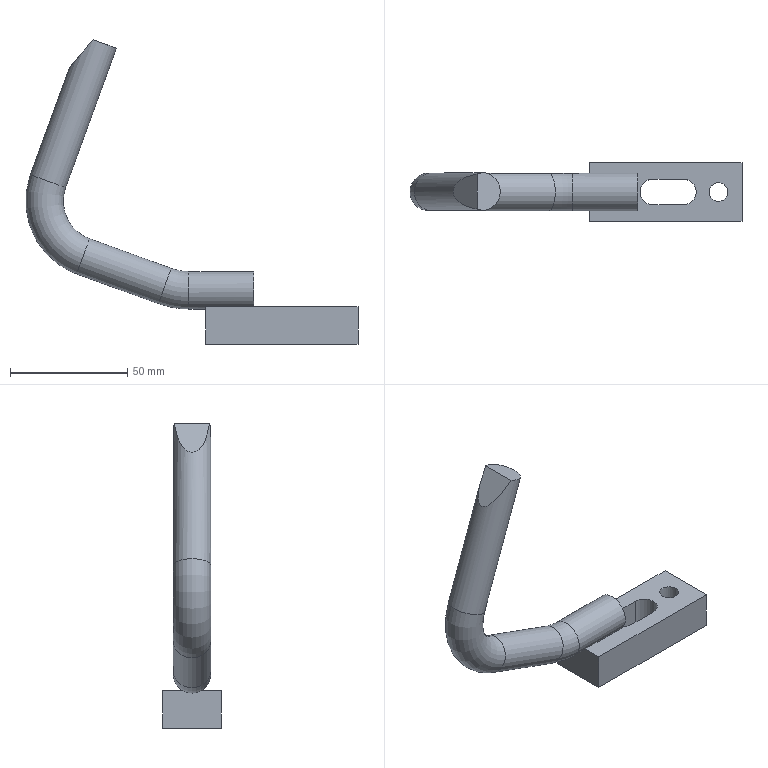Part | NX | features MAIN_BODY 2 | 1 solid | 19 faces | box 141.738 x 25 x 129.841 mm | volume 56656 mm3 | plane 10 | cylinder 6 | torus 2 | spline 1 | commonest cylinder face diameters 16 x3 11 x2 8 x1
STEP:
#1=CARTESIAN_POINT('',(970.,-301.373,-139.));
#2=VERTEX_POINT('',#1);
#3=CARTESIAN_POINT('',(970.,-293.627,-139.));
#4=VERTEX_POINT('',#3);
#5=CARTESIAN_POINT('',(970.,-297.5,-132.));
#6=DIRECTION('',(-1.,0.,0.));
#7=DIRECTION('',(0.,-1.,0.));
#8=AXIS2_PLACEMENT_3D('',#5,#6,#7);
#9=CIRCLE('',#8,8.);
#10=EDGE_CURVE('',#2,#4,#9,.F.);
#11=ORIENTED_EDGE('',*,*,#10,.T.);
#12=CARTESIAN_POINT('',(970.,-285.,-139.));
#13=VERTEX_POINT('',#12);
#14=CARTESIAN_POINT('',(970.,-285.5,-139.));
#15=DIRECTION('',(0.,1.,0.));
#16=VECTOR('',#15,1000.);
#17=LINE('',#14,#16);
#18=EDGE_CURVE('',#13,#4,#17,.F.);
#19=ORIENTED_EDGE('',*,*,#18,.F.);
#20=CARTESIAN_POINT('',(970.,-285.,-155.));
#21=VERTEX_POINT('',#20);
#22=CARTESIAN_POINT('',(970.,-285.,-135.));
#23=DIRECTION('',(0.,0.,-1.));
#24=VECTOR('',#23,1000.);
#25=LINE('',#22,#24);
#26=EDGE_CURVE('',#21,#13,#25,.F.);
#27=ORIENTED_EDGE('',*,*,#26,.F.);
#28=CARTESIAN_POINT('',(970.,-310.,-155.));
#29=VERTEX_POINT('',#28);
#30=CARTESIAN_POINT('',(970.,-285.5,-155.));
#31=DIRECTION('',(0.,1.,0.));
#32=VECTOR('',#31,1000.);
#33=LINE('',#30,#32);
#34=EDGE_CURVE('',#21,#29,#33,.F.);
#35=ORIENTED_EDGE('',*,*,#34,.T.);
#36=CARTESIAN_POINT('',(970.,-310.,-139.));
#37=VERTEX_POINT('',#36);
#38=CARTESIAN_POINT('',(970.,-310.,-135.));
#39=DIRECTION('',(0.,0.,1.));
#40=VECTOR('',#39,1000.);
#41=LINE('',#38,#40);
#42=EDGE_CURVE('',#29,#37,#41,.T.);
#43=ORIENTED_EDGE('',*,*,#42,.T.);
#44=CARTESIAN_POINT('',(970.,-285.5,-139.));
#45=DIRECTION('',(0.,1.,0.));
#46=VECTOR('',#45,1000.);
#47=LINE('',#44,#46);
#48=EDGE_CURVE('',#2,#37,#47,.F.);
#49=ORIENTED_EDGE('',*,*,#48,.F.);
#50=EDGE_LOOP('',(#11,#19,#27,#35,#43,#49));
#51=FACE_BOUND('',#50,.T.);
#52=CARTESIAN_POINT('',(970.,-285.5,-135.));
#53=DIRECTION('',(1.,0.,0.));
#54=DIRECTION('',(0.,-1.,0.));
#55=AXIS2_PLACEMENT_3D('',#52,#53,#54);
#56=PLANE('',#55);
#57=ADVANCED_FACE('',(#51),#56,.F.);
#58=ORIENTED_EDGE('',*,*,#48,.T.);
#59=CARTESIAN_POINT('',(1035.,-310.,-139.));
#60=VERTEX_POINT('',#59);
#61=CARTESIAN_POINT('',(900.,-310.,-139.));
#62=DIRECTION('',(-1.,0.,0.));
#63=VECTOR('',#62,1000.);
#64=LINE('',#61,#63);
#65=EDGE_CURVE('',#37,#60,#64,.F.);
#66=ORIENTED_EDGE('',*,*,#65,.T.);
#67=CARTESIAN_POINT('',(1035.,-285.,-139.));
#68=VERTEX_POINT('',#67);
#69=CARTESIAN_POINT('',(1035.,-285.5,-139.));
#70=DIRECTION('',(0.,-1.,0.));
#71=VECTOR('',#70,1000.);
#72=LINE('',#69,#71);
#73=EDGE_CURVE('',#68,#60,#72,.T.);
#74=ORIENTED_EDGE('',*,*,#73,.F.);
#75=CARTESIAN_POINT('',(900.,-285.,-139.));
#76=DIRECTION('',(1.,0.,0.));
#77=VECTOR('',#76,1000.);
#78=LINE('',#75,#77);
#79=EDGE_CURVE('',#13,#68,#78,.T.);
#80=ORIENTED_EDGE('',*,*,#79,.F.);
#81=ORIENTED_EDGE('',*,*,#18,.T.);
#82=CARTESIAN_POINT('',(990.552,-293.627,-139.));
#83=VERTEX_POINT('',#82);
#84=CARTESIAN_POINT('',(962.842,-293.627,-139.));
#85=DIRECTION('',(1.,0.,0.));
#86=VECTOR('',#85,1000.);
#87=LINE('',#84,#86);
#88=EDGE_CURVE('',#83,#4,#87,.F.);
#89=ORIENTED_EDGE('',*,*,#88,.F.);
#90=CARTESIAN_POINT('',(990.552,-301.373,-139.));
#91=VERTEX_POINT('',#90);
#92=CARTESIAN_POINT('',(990.552,-285.5,-139.));
#93=DIRECTION('',(0.,1.,0.));
#94=VECTOR('',#93,1000.);
#95=LINE('',#92,#94);
#96=EDGE_CURVE('',#91,#83,#95,.T.);
#97=ORIENTED_EDGE('',*,*,#96,.F.);
#98=CARTESIAN_POINT('',(962.842,-301.373,-139.));
#99=DIRECTION('',(1.,0.,0.));
#100=VECTOR('',#99,1000.);
#101=LINE('',#98,#100);
#102=EDGE_CURVE('',#2,#91,#101,.T.);
#103=ORIENTED_EDGE('',*,*,#102,.F.);
#104=EDGE_LOOP('',(#58,#66,#74,#80,#81,#89,#97,#103));
#105=FACE_BOUND('',#104,.T.);
#106=CARTESIAN_POINT('',(1021.,-297.5,-139.));
#107=VERTEX_POINT('',#106);
#108=CARTESIAN_POINT('',(1025.,-297.5,-139.));
#109=DIRECTION('',(0.,0.,1.));
#110=DIRECTION('',(-1.,0.,0.));
#111=AXIS2_PLACEMENT_3D('',#108,#109,#110);
#112=CIRCLE('',#111,4.);
#113=EDGE_CURVE('',#107,#107,#112,.F.);
#114=ORIENTED_EDGE('',*,*,#113,.T.);
#115=EDGE_LOOP('',(#114));
#116=FACE_BOUND('',#115,.T.);
#117=CARTESIAN_POINT('',(1010.,-292.,-139.));
#118=VERTEX_POINT('',#117);
#119=CARTESIAN_POINT('',(1010.,-303.,-139.));
#120=VERTEX_POINT('',#119);
#121=CARTESIAN_POINT('',(1010.,-297.5,-139.));
#122=DIRECTION('',(0.,0.,1.));
#123=DIRECTION('',(-1.,0.,0.));
#124=AXIS2_PLACEMENT_3D('',#121,#122,#123);
#125=CIRCLE('',#124,5.5);
#126=EDGE_CURVE('',#118,#120,#125,.F.);
#127=ORIENTED_EDGE('',*,*,#126,.T.);
#128=CARTESIAN_POINT('',(997.,-303.,-139.));
#129=VERTEX_POINT('',#128);
#130=CARTESIAN_POINT('',(969.,-303.,-139.));
#131=DIRECTION('',(-1.,0.,0.));
#132=VECTOR('',#131,1000.);
#133=LINE('',#130,#132);
#134=EDGE_CURVE('',#120,#129,#133,.T.);
#135=ORIENTED_EDGE('',*,*,#134,.T.);
#136=CARTESIAN_POINT('',(997.,-292.,-139.));
#137=VERTEX_POINT('',#136);
#138=CARTESIAN_POINT('',(997.,-297.5,-139.));
#139=DIRECTION('',(0.,0.,1.));
#140=DIRECTION('',(-1.,0.,0.));
#141=AXIS2_PLACEMENT_3D('',#138,#139,#140);
#142=CIRCLE('',#141,5.5);
#143=EDGE_CURVE('',#129,#137,#142,.F.);
#144=ORIENTED_EDGE('',*,*,#143,.T.);
#145=CARTESIAN_POINT('',(969.,-292.,-139.));
#146=DIRECTION('',(-1.,0.,0.));
#147=VECTOR('',#146,1000.);
#148=LINE('',#145,#147);
#149=EDGE_CURVE('',#137,#118,#148,.F.);
#150=ORIENTED_EDGE('',*,*,#149,.T.);
#151=EDGE_LOOP('',(#127,#135,#144,#150));
#152=FACE_BOUND('',#151,.T.);
#153=CARTESIAN_POINT('',(900.,-285.5,-139.));
#154=DIRECTION('',(0.,0.,-1.));
#155=DIRECTION('',(-1.,0.,0.));
#156=AXIS2_PLACEMENT_3D('',#153,#154,#155);
#157=PLANE('',#156);
#158=ADVANCED_FACE('',(#105,#116,#152),#157,.F.);
#159=CARTESIAN_POINT('',(1035.,-285.,-155.));
#160=VERTEX_POINT('',#159);
#161=CARTESIAN_POINT('',(1035.,-285.,-135.));
#162=DIRECTION('',(0.,0.,1.));
#163=VECTOR('',#162,1000.);
#164=LINE('',#161,#163);
#165=EDGE_CURVE('',#160,#68,#164,.T.);
#166=ORIENTED_EDGE('',*,*,#165,.F.);
#167=CARTESIAN_POINT('',(900.,-285.,-155.));
#168=DIRECTION('',(1.,0.,0.));
#169=VECTOR('',#168,1000.);
#170=LINE('',#167,#169);
#171=EDGE_CURVE('',#21,#160,#170,.T.);
#172=ORIENTED_EDGE('',*,*,#171,.F.);
#173=ORIENTED_EDGE('',*,*,#26,.T.);
#174=ORIENTED_EDGE('',*,*,#79,.T.);
#175=EDGE_LOOP('',(#166,#172,#173,#174));
#176=FACE_BOUND('',#175,.T.);
#177=CARTESIAN_POINT('',(900.,-285.,-135.));
#178=DIRECTION('',(0.,1.,0.));
#179=DIRECTION('',(1.,0.,0.));
#180=AXIS2_PLACEMENT_3D('',#177,#178,#179);
#181=PLANE('',#180);
#182=ADVANCED_FACE('',(#176),#181,.T.);
#183=ORIENTED_EDGE('',*,*,#42,.F.);
#184=CARTESIAN_POINT('',(1035.,-310.,-155.));
#185=VERTEX_POINT('',#184);
#186=CARTESIAN_POINT('',(900.,-310.,-155.));
#187=DIRECTION('',(-1.,0.,0.));
#188=VECTOR('',#187,1000.);
#189=LINE('',#186,#188);
#190=EDGE_CURVE('',#29,#185,#189,.F.);
#191=ORIENTED_EDGE('',*,*,#190,.T.);
#192=CARTESIAN_POINT('',(1035.,-310.,-135.));
#193=DIRECTION('',(0.,0.,-1.));
#194=VECTOR('',#193,1000.);
#195=LINE('',#192,#194);
#196=EDGE_CURVE('',#185,#60,#195,.F.);
#197=ORIENTED_EDGE('',*,*,#196,.T.);
#198=ORIENTED_EDGE('',*,*,#65,.F.);
#199=EDGE_LOOP('',(#183,#191,#197,#198));
#200=FACE_BOUND('',#199,.T.);
#201=CARTESIAN_POINT('',(900.,-310.,-135.));
#202=DIRECTION('',(0.,1.,0.));
#203=DIRECTION('',(1.,0.,0.));
#204=AXIS2_PLACEMENT_3D('',#201,#202,#203);
#205=PLANE('',#204);
#206=ADVANCED_FACE('',(#200),#205,.F.);
#207=CARTESIAN_POINT('',(1035.,-285.5,-155.));
#208=DIRECTION('',(0.,-1.,0.));
#209=VECTOR('',#208,1000.);
#210=LINE('',#207,#209);
#211=EDGE_CURVE('',#160,#185,#210,.T.);
#212=ORIENTED_EDGE('',*,*,#211,.F.);
#213=ORIENTED_EDGE('',*,*,#165,.T.);
#214=ORIENTED_EDGE('',*,*,#73,.T.);
#215=ORIENTED_EDGE('',*,*,#196,.F.);
#216=EDGE_LOOP('',(#212,#213,#214,#215));
#217=FACE_BOUND('',#216,.T.);
#218=CARTESIAN_POINT('',(1035.,-285.5,-135.));
#219=DIRECTION('',(1.,0.,0.));
#220=DIRECTION('',(0.,-1.,0.));
#221=AXIS2_PLACEMENT_3D('',#218,#219,#220);
#222=PLANE('',#221);
#223=ADVANCED_FACE('',(#217),#222,.T.);
#224=CARTESIAN_POINT('',(1021.03,-297.987,-155.));
#225=VERTEX_POINT('',#224);
#226=CARTESIAN_POINT('',(1025.,-297.5,-155.));
#227=DIRECTION('',(0.,0.,-1.));
#228=DIRECTION('',(-0.9925,-0.1219,0.));
#229=AXIS2_PLACEMENT_3D('',#226,#227,#228);
#230=CIRCLE('',#229,4.);
#231=EDGE_CURVE('',#225,#225,#230,.T.);
#232=ORIENTED_EDGE('',*,*,#231,.F.);
#233=EDGE_LOOP('',(#232));
#234=FACE_BOUND('',#233,.T.);
#235=CARTESIAN_POINT('',(1010.,-303.,-155.));
#236=VERTEX_POINT('',#235);
#237=CARTESIAN_POINT('',(997.,-303.,-155.));
#238=VERTEX_POINT('',#237);
#239=CARTESIAN_POINT('',(969.,-303.,-155.));
#240=DIRECTION('',(-1.,0.,0.));
#241=VECTOR('',#240,1000.);
#242=LINE('',#239,#241);
#243=EDGE_CURVE('',#236,#238,#242,.T.);
#244=ORIENTED_EDGE('',*,*,#243,.F.);
#245=CARTESIAN_POINT('',(1010.,-292.,-155.));
#246=VERTEX_POINT('',#245);
#247=CARTESIAN_POINT('',(1010.,-297.5,-155.));
#248=DIRECTION('',(0.,0.,1.));
#249=DIRECTION('',(-0.9925,-0.1219,0.));
#250=AXIS2_PLACEMENT_3D('',#247,#248,#249);
#251=CIRCLE('',#250,5.5);
#252=EDGE_CURVE('',#246,#236,#251,.F.);
#253=ORIENTED_EDGE('',*,*,#252,.F.);
#254=CARTESIAN_POINT('',(997.,-292.,-155.));
#255=VERTEX_POINT('',#254);
#256=CARTESIAN_POINT('',(969.,-292.,-155.));
#257=DIRECTION('',(-1.,0.,0.));
#258=VECTOR('',#257,1000.);
#259=LINE('',#256,#258);
#260=EDGE_CURVE('',#255,#246,#259,.F.);
#261=ORIENTED_EDGE('',*,*,#260,.F.);
#262=CARTESIAN_POINT('',(997.,-297.5,-155.));
#263=DIRECTION('',(0.,0.,1.));
#264=DIRECTION('',(-0.9925,-0.1219,0.));
#265=AXIS2_PLACEMENT_3D('',#262,#263,#264);
#266=CIRCLE('',#265,5.5);
#267=EDGE_CURVE('',#238,#255,#266,.F.);
#268=ORIENTED_EDGE('',*,*,#267,.F.);
#269=EDGE_LOOP('',(#244,#253,#261,#268));
#270=FACE_BOUND('',#269,.T.);
#271=ORIENTED_EDGE('',*,*,#190,.F.);
#272=ORIENTED_EDGE('',*,*,#34,.F.);
#273=ORIENTED_EDGE('',*,*,#171,.T.);
#274=ORIENTED_EDGE('',*,*,#211,.T.);
#275=EDGE_LOOP('',(#271,#272,#273,#274));
#276=FACE_BOUND('',#275,.T.);
#277=CARTESIAN_POINT('',(900.,-285.5,-155.));
#278=DIRECTION('',(0.,0.,-1.));
#279=DIRECTION('',(-1.,0.,0.));
#280=AXIS2_PLACEMENT_3D('',#277,#278,#279);
#281=PLANE('',#280);
#282=ADVANCED_FACE('',(#234,#270,#276),#281,.T.);
#283=ORIENTED_EDGE('',*,*,#143,.F.);
#284=CARTESIAN_POINT('',(997.,-303.,-119.));
#285=DIRECTION('',(0.,0.,-1.));
#286=VECTOR('',#285,1000.);
#287=LINE('',#284,#286);
#288=EDGE_CURVE('',#129,#238,#287,.T.);
#289=ORIENTED_EDGE('',*,*,#288,.T.);
#290=ORIENTED_EDGE('',*,*,#267,.T.);
#291=CARTESIAN_POINT('',(997.,-292.,-119.));
#292=DIRECTION('',(0.,0.,-1.));
#293=VECTOR('',#292,1000.);
#294=LINE('',#291,#293);
#295=EDGE_CURVE('',#137,#255,#294,.T.);
#296=ORIENTED_EDGE('',*,*,#295,.F.);
#297=EDGE_LOOP('',(#283,#289,#290,#296));
#298=FACE_BOUND('',#297,.T.);
#299=CARTESIAN_POINT('',(997.,-297.5,-119.));
#300=DIRECTION('',(0.,0.,-1.));
#301=DIRECTION('',(-1.,0.,0.));
#302=AXIS2_PLACEMENT_3D('',#299,#300,#301);
#303=CYLINDRICAL_SURFACE('',#302,5.5);
#304=ADVANCED_FACE('',(#298),#303,.F.);
#305=ORIENTED_EDGE('',*,*,#126,.F.);
#306=CARTESIAN_POINT('',(1010.,-292.,-119.));
#307=DIRECTION('',(0.,0.,-1.));
#308=VECTOR('',#307,1000.);
#309=LINE('',#306,#308);
#310=EDGE_CURVE('',#118,#246,#309,.T.);
#311=ORIENTED_EDGE('',*,*,#310,.T.);
#312=ORIENTED_EDGE('',*,*,#252,.T.);
#313=CARTESIAN_POINT('',(1010.,-303.,-119.));
#314=DIRECTION('',(0.,0.,-1.));
#315=VECTOR('',#314,1000.);
#316=LINE('',#313,#315);
#317=EDGE_CURVE('',#120,#236,#316,.T.);
#318=ORIENTED_EDGE('',*,*,#317,.F.);
#319=EDGE_LOOP('',(#305,#311,#312,#318));
#320=FACE_BOUND('',#319,.T.);
#321=CARTESIAN_POINT('',(1010.,-297.5,-119.));
#322=DIRECTION('',(0.,0.,-1.));
#323=DIRECTION('',(-1.,0.,0.));
#324=AXIS2_PLACEMENT_3D('',#321,#322,#323);
#325=CYLINDRICAL_SURFACE('',#324,5.5);
#326=ADVANCED_FACE('',(#320),#325,.F.);
#327=ORIENTED_EDGE('',*,*,#317,.T.);
#328=ORIENTED_EDGE('',*,*,#243,.T.);
#329=ORIENTED_EDGE('',*,*,#288,.F.);
#330=ORIENTED_EDGE('',*,*,#134,.F.);
#331=EDGE_LOOP('',(#327,#328,#329,#330));
#332=FACE_BOUND('',#331,.T.);
#333=CARTESIAN_POINT('',(969.,-303.,-119.));
#334=DIRECTION('',(0.,-1.,0.));
#335=DIRECTION('',(-1.,0.,0.));
#336=AXIS2_PLACEMENT_3D('',#333,#334,#335);
#337=PLANE('',#336);
#338=ADVANCED_FACE('',(#332),#337,.F.);
#339=ORIENTED_EDGE('',*,*,#295,.T.);
#340=ORIENTED_EDGE('',*,*,#260,.T.);
#341=ORIENTED_EDGE('',*,*,#310,.F.);
#342=ORIENTED_EDGE('',*,*,#149,.F.);
#343=EDGE_LOOP('',(#339,#340,#341,#342));
#344=FACE_BOUND('',#343,.T.);
#345=CARTESIAN_POINT('',(969.,-292.,-119.));
#346=DIRECTION('',(0.,-1.,0.));
#347=DIRECTION('',(-1.,0.,0.));
#348=AXIS2_PLACEMENT_3D('',#345,#346,#347);
#349=PLANE('',#348);
#350=ADVANCED_FACE('',(#344),#349,.T.);
#351=ORIENTED_EDGE('',*,*,#231,.T.);
#352=EDGE_LOOP('',(#351));
#353=FACE_BOUND('',#352,.T.);
#354=ORIENTED_EDGE('',*,*,#113,.F.);
#355=EDGE_LOOP('',(#354));
#356=FACE_BOUND('',#355,.T.);
#357=CARTESIAN_POINT('',(1025.,-297.5,-139.));
#358=DIRECTION('',(0.,0.,-1.));
#359=DIRECTION('',(-0.9925,-0.1219,0.));
#360=AXIS2_PLACEMENT_3D('',#357,#358,#359);
#361=CYLINDRICAL_SURFACE('',#360,4.);
#362=ADVANCED_FACE('',(#353,#356),#361,.F.);
#363=CARTESIAN_POINT('',(962.842,-297.5,-140.));
#364=VERTEX_POINT('',#363);
#365=CARTESIAN_POINT('',(962.842,-297.5,-132.));
#366=DIRECTION('',(-1.,0.,0.));
#367=DIRECTION('',(0.,0.,-1.));
#368=AXIS2_PLACEMENT_3D('',#365,#366,#367);
#369=CIRCLE('',#368,8.);
#370=EDGE_CURVE('',#364,#364,#369,.T.);
#371=ORIENTED_EDGE('',*,*,#370,.F.);
#372=EDGE_LOOP('',(#371));
#373=FACE_BOUND('',#372,.T.);
#374=ORIENTED_EDGE('',*,*,#102,.T.);
#375=CARTESIAN_POINT('',(990.552,-297.5,-132.));
#376=DIRECTION('',(-1.,0.,0.));
#377=DIRECTION('',(0.,0.,-1.));
#378=AXIS2_PLACEMENT_3D('',#375,#376,#377);
#379=CIRCLE('',#378,8.);
#380=EDGE_CURVE('',#91,#83,#379,.T.);
#381=ORIENTED_EDGE('',*,*,#380,.T.);
#382=ORIENTED_EDGE('',*,*,#88,.T.);
#383=ORIENTED_EDGE('',*,*,#10,.F.);
#384=EDGE_LOOP('',(#374,#381,#382,#383));
#385=FACE_BOUND('',#384,.T.);
#386=CARTESIAN_POINT('',(962.842,-297.5,-132.));
#387=DIRECTION('',(1.,0.,0.));
#388=DIRECTION('',(0.,0.,-1.));
#389=AXIS2_PLACEMENT_3D('',#386,#387,#388);
#390=CYLINDRICAL_SURFACE('',#389,8.);
#391=ADVANCED_FACE('',(#373,#385),#390,.T.);
#392=ORIENTED_EDGE('',*,*,#96,.T.);
#393=ORIENTED_EDGE('',*,*,#380,.F.);
#394=EDGE_LOOP('',(#392,#393));
#395=FACE_BOUND('',#394,.T.);
#396=CARTESIAN_POINT('',(990.552,-297.5,-132.));
#397=DIRECTION('',(1.,0.,0.));
#398=DIRECTION('',(0.,0.,-1.));
#399=AXIS2_PLACEMENT_3D('',#396,#397,#398);
#400=PLANE('',#399);
#401=ADVANCED_FACE('',(#395),#400,.T.);
#402=CARTESIAN_POINT('',(895.252,-297.5,-82.72));
#403=VERTEX_POINT('',#402);
#404=CARTESIAN_POINT('',(902.769,-297.5,-85.456));
#405=DIRECTION('',(0.342,0.,0.9397));
#406=DIRECTION('',(-0.9397,0.,0.342));
#407=AXIS2_PLACEMENT_3D('',#404,#405,#406);
#408=CIRCLE('',#407,8.);
#409=EDGE_CURVE('',#403,#403,#408,.T.);
#410=ORIENTED_EDGE('',*,*,#409,.T.);
#411=EDGE_LOOP('',(#410));
#412=FACE_BOUND('',#411,.T.);
#413=CARTESIAN_POINT('',(921.975,-305.074,-25.159));
#414=VERTEX_POINT('',#413);
#415=CARTESIAN_POINT('',(921.975,-289.926,-25.159));
#416=VERTEX_POINT('',#415);
#417=CARTESIAN_POINT('',(924.395,-297.5,-26.04));
#418=DIRECTION('',(0.342,0.,0.9397));
#419=DIRECTION('',(-0.9397,0.,0.342));
#420=AXIS2_PLACEMENT_3D('',#417,#418,#419);
#421=CIRCLE('',#420,8.);
#422=EDGE_CURVE('',#414,#416,#421,.T.);
#423=ORIENTED_EDGE('',*,*,#422,.F.);
#424=CARTESIAN_POINT('',(921.975,-289.926,-25.159));
#425=CARTESIAN_POINT('',(920.983,-290.105,-26.342));
#426=CARTESIAN_POINT('',(919.015,-290.582,-28.686));
#427=CARTESIAN_POINT('',(916.59,-291.561,-31.577));
#428=CARTESIAN_POINT('',(914.734,-292.685,-33.788));
#429=CARTESIAN_POINT('',(913.406,-293.799,-35.371));
#430=CARTESIAN_POINT('',(912.229,-295.253,-36.773));
#431=CARTESIAN_POINT('',(911.548,-297.538,-37.585));
#432=CARTESIAN_POINT('',(912.262,-299.8,-36.734));
#433=CARTESIAN_POINT('',(913.447,-301.242,-35.323));
#434=CARTESIAN_POINT('',(914.775,-302.342,-33.739));
#435=CARTESIAN_POINT('',(916.614,-303.449,-31.547));
#436=CARTESIAN_POINT('',(919.022,-304.419,-28.679));
#437=CARTESIAN_POINT('',(920.987,-304.895,-26.336));
#438=CARTESIAN_POINT('',(921.975,-305.074,-25.159));
#439=B_SPLINE_CURVE_WITH_KNOTS('',3,(#424,#425,#426,#427,#428,#429,#430,#431,#432,#433,#434,#435,#436,#437,#438),.UNSPECIFIED.,.F.,.F.,(4,1,1,1,1,1,1,1,1,1,1,1,4),(0.,0.004649,0.009299,0.01162,0.01395,0.01627,0.0186,0.02092,0.02325,0.02557,0.0279,0.03255,0.03719),.UNSPECIFIED.);
#440=EDGE_CURVE('',#416,#414,#439,.T.);
#441=ORIENTED_EDGE('',*,*,#440,.F.);
#442=EDGE_LOOP('',(#423,#441));
#443=FACE_BOUND('',#442,.T.);
#444=CARTESIAN_POINT('',(902.769,-297.5,-85.456));
#445=DIRECTION('',(0.342,0.,0.9397));
#446=DIRECTION('',(0.9397,0.,-0.342));
#447=AXIS2_PLACEMENT_3D('',#444,#445,#446);
#448=CYLINDRICAL_SURFACE('',#447,8.);
#449=ADVANCED_FACE('',(#412,#443),#448,.T.);
#450=CARTESIAN_POINT('',(914.975,-297.5,-125.017));
#451=VERTEX_POINT('',#450);
#452=CARTESIAN_POINT('',(917.711,-297.5,-117.499));
#453=DIRECTION('',(-0.9397,0.,0.342));
#454=DIRECTION('',(-0.342,0.,-0.9397));
#455=AXIS2_PLACEMENT_3D('',#452,#453,#454);
#456=CIRCLE('',#455,8.);
#457=EDGE_CURVE('',#451,#451,#456,.T.);
#458=ORIENTED_EDGE('',*,*,#457,.T.);
#459=EDGE_LOOP('',(#458));
#460=FACE_BOUND('',#459,.T.);
#461=ORIENTED_EDGE('',*,*,#409,.F.);
#462=EDGE_LOOP('',(#461));
#463=FACE_BOUND('',#462,.T.);
#464=CARTESIAN_POINT('',(926.262,-297.5,-94.007));
#465=DIRECTION('',(0.,-1.,0.));
#466=DIRECTION('',(0.,0.,1.));
#467=AXIS2_PLACEMENT_3D('',#464,#465,#466);
#468=TOROIDAL_SURFACE('',#467,25.,8.);
#469=ADVANCED_FACE('',(#460,#463),#468,.T.);
#470=CARTESIAN_POINT('',(949.845,-297.5,-137.708));
#471=VERTEX_POINT('',#470);
#472=CARTESIAN_POINT('',(952.581,-297.5,-130.191));
#473=DIRECTION('',(-0.9397,0.,0.342));
#474=DIRECTION('',(-0.342,0.,-0.9397));
#475=AXIS2_PLACEMENT_3D('',#472,#473,#474);
#476=CIRCLE('',#475,8.);
#477=EDGE_CURVE('',#471,#471,#476,.T.);
#478=ORIENTED_EDGE('',*,*,#477,.T.);
#479=EDGE_LOOP('',(#478));
#480=FACE_BOUND('',#479,.T.);
#481=ORIENTED_EDGE('',*,*,#457,.F.);
#482=EDGE_LOOP('',(#481));
#483=FACE_BOUND('',#482,.T.);
#484=CARTESIAN_POINT('',(952.581,-297.5,-130.191));
#485=DIRECTION('',(-0.9397,0.,0.342));
#486=DIRECTION('',(0.342,0.,0.9397));
#487=AXIS2_PLACEMENT_3D('',#484,#485,#486);
#488=CYLINDRICAL_SURFACE('',#487,8.);
#489=ADVANCED_FACE('',(#480,#483),#488,.T.);
#490=ORIENTED_EDGE('',*,*,#370,.T.);
#491=EDGE_LOOP('',(#490));
#492=FACE_BOUND('',#491,.T.);
#493=ORIENTED_EDGE('',*,*,#477,.F.);
#494=EDGE_LOOP('',(#493));
#495=FACE_BOUND('',#494,.T.);
#496=CARTESIAN_POINT('',(962.842,-297.5,-102.));
#497=DIRECTION('',(0.,-1.,0.));
#498=DIRECTION('',(0.,0.,1.));
#499=AXIS2_PLACEMENT_3D('',#496,#497,#498);
#500=TOROIDAL_SURFACE('',#499,30.,8.);
#501=ADVANCED_FACE('',(#492,#495),#500,.T.);
#502=ORIENTED_EDGE('',*,*,#422,.T.);
#503=CARTESIAN_POINT('',(921.975,-305.074,-25.159));
#504=CARTESIAN_POINT('',(921.975,-300.025,-25.159));
#505=CARTESIAN_POINT('',(921.975,-294.975,-25.159));
#506=CARTESIAN_POINT('',(921.975,-289.926,-25.159));
#507=B_SPLINE_CURVE_WITH_KNOTS('',3,(#503,#504,#505,#506),.UNSPECIFIED.,.F.,.F.,(4,4),(0.01671,0.03186),.UNSPECIFIED.);
#508=EDGE_CURVE('',#414,#416,#507,.T.);
#509=ORIENTED_EDGE('',*,*,#508,.F.);
#510=EDGE_LOOP('',(#502,#509));
#511=FACE_BOUND('',#510,.T.);
#512=CARTESIAN_POINT('',(924.395,-297.5,-26.04));
#513=DIRECTION('',(-0.342,0.,-0.9397));
#514=DIRECTION('',(-0.9397,0.,0.342));
#515=AXIS2_PLACEMENT_3D('',#512,#513,#514);
#516=PLANE('',#515);
#517=ADVANCED_FACE('',(#511),#516,.F.);
#518=ORIENTED_EDGE('',*,*,#508,.T.);
#519=ORIENTED_EDGE('',*,*,#440,.T.);
#520=EDGE_LOOP('',(#518,#519));
#521=FACE_BOUND('',#520,.T.);
#522=CARTESIAN_POINT('',(921.975,-289.835,-25.159));
#523=CARTESIAN_POINT('',(921.975,-294.945,-25.159));
#524=CARTESIAN_POINT('',(921.975,-300.055,-25.159));
#525=CARTESIAN_POINT('',(921.975,-305.165,-25.159));
#526=CARTESIAN_POINT('',(918.552,-289.835,-29.238));
#527=CARTESIAN_POINT('',(918.552,-294.945,-29.238));
#528=CARTESIAN_POINT('',(918.552,-300.055,-29.238));
#529=CARTESIAN_POINT('',(918.552,-305.165,-29.238));
#530=CARTESIAN_POINT('',(915.129,-289.835,-33.318));
#531=CARTESIAN_POINT('',(915.129,-294.945,-33.318));
#532=CARTESIAN_POINT('',(915.129,-300.055,-33.318));
#533=CARTESIAN_POINT('',(915.129,-305.165,-33.318));
#534=CARTESIAN_POINT('',(911.706,-289.835,-37.398));
#535=CARTESIAN_POINT('',(911.706,-294.945,-37.398));
#536=CARTESIAN_POINT('',(911.706,-300.055,-37.398));
#537=CARTESIAN_POINT('',(911.706,-305.165,-37.398));
#538=B_SPLINE_SURFACE_WITH_KNOTS('',3,3,((#522,#523,#524,#525),(#526,#527,#528,#529),(#530,#531,#532,#533),(#534,#535,#536,#537)),.UNSPECIFIED.,.F.,.F.,.F.,(4,4),(4,4),(0.4789,0.7052),(0.3422,0.6578),.UNSPECIFIED.);
#539=ADVANCED_FACE('',(#521),#538,.T.);
#540=CLOSED_SHELL('',(#57,#158,#182,#206,#223,#282,#304,#326,#338,#350,#362,#391,#401,#449,#469,#489,#501,#517,#539));
#541=MANIFOLD_SOLID_BREP('',#540);
#542=(LENGTH_UNIT()NAMED_UNIT(*)SI_UNIT(.MILLI.,.METRE.));
#543=UNCERTAINTY_MEASURE_WITH_UNIT(LENGTH_MEASURE(0.0508),#542,'','');
#544=(NAMED_UNIT(*)PLANE_ANGLE_UNIT()SI_UNIT($,.RADIAN.));
#545=(NAMED_UNIT(*)SI_UNIT($,.STERADIAN.)SOLID_ANGLE_UNIT());
#546=(GEOMETRIC_REPRESENTATION_CONTEXT(3)GLOBAL_UNCERTAINTY_ASSIGNED_CONTEXT((#543))GLOBAL_UNIT_ASSIGNED_CONTEXT((#542,#544,#545))REPRESENTATION_CONTEXT('',''));
#547=ADVANCED_BREP_SHAPE_REPRESENTATION('',(#541),#546);